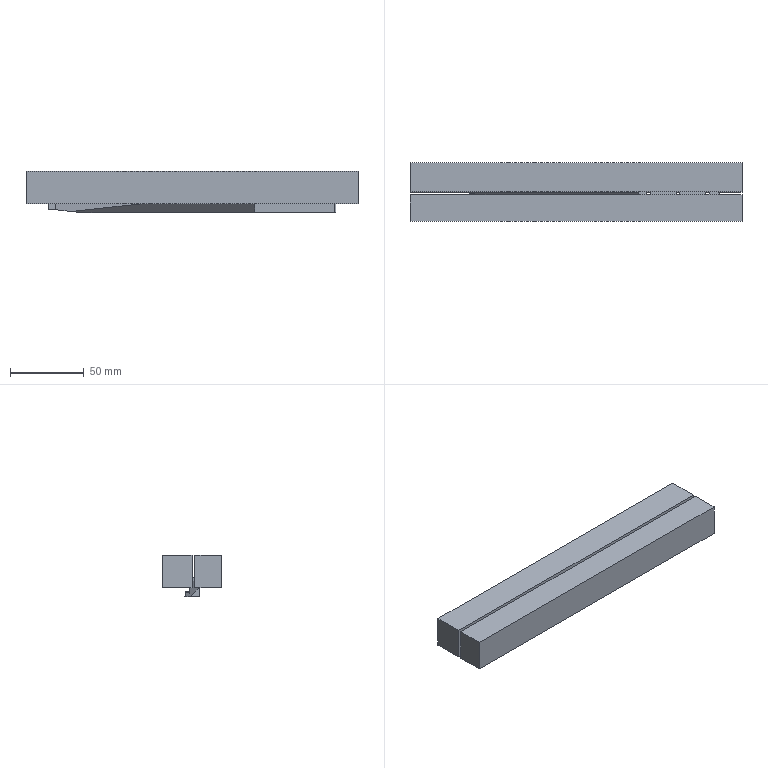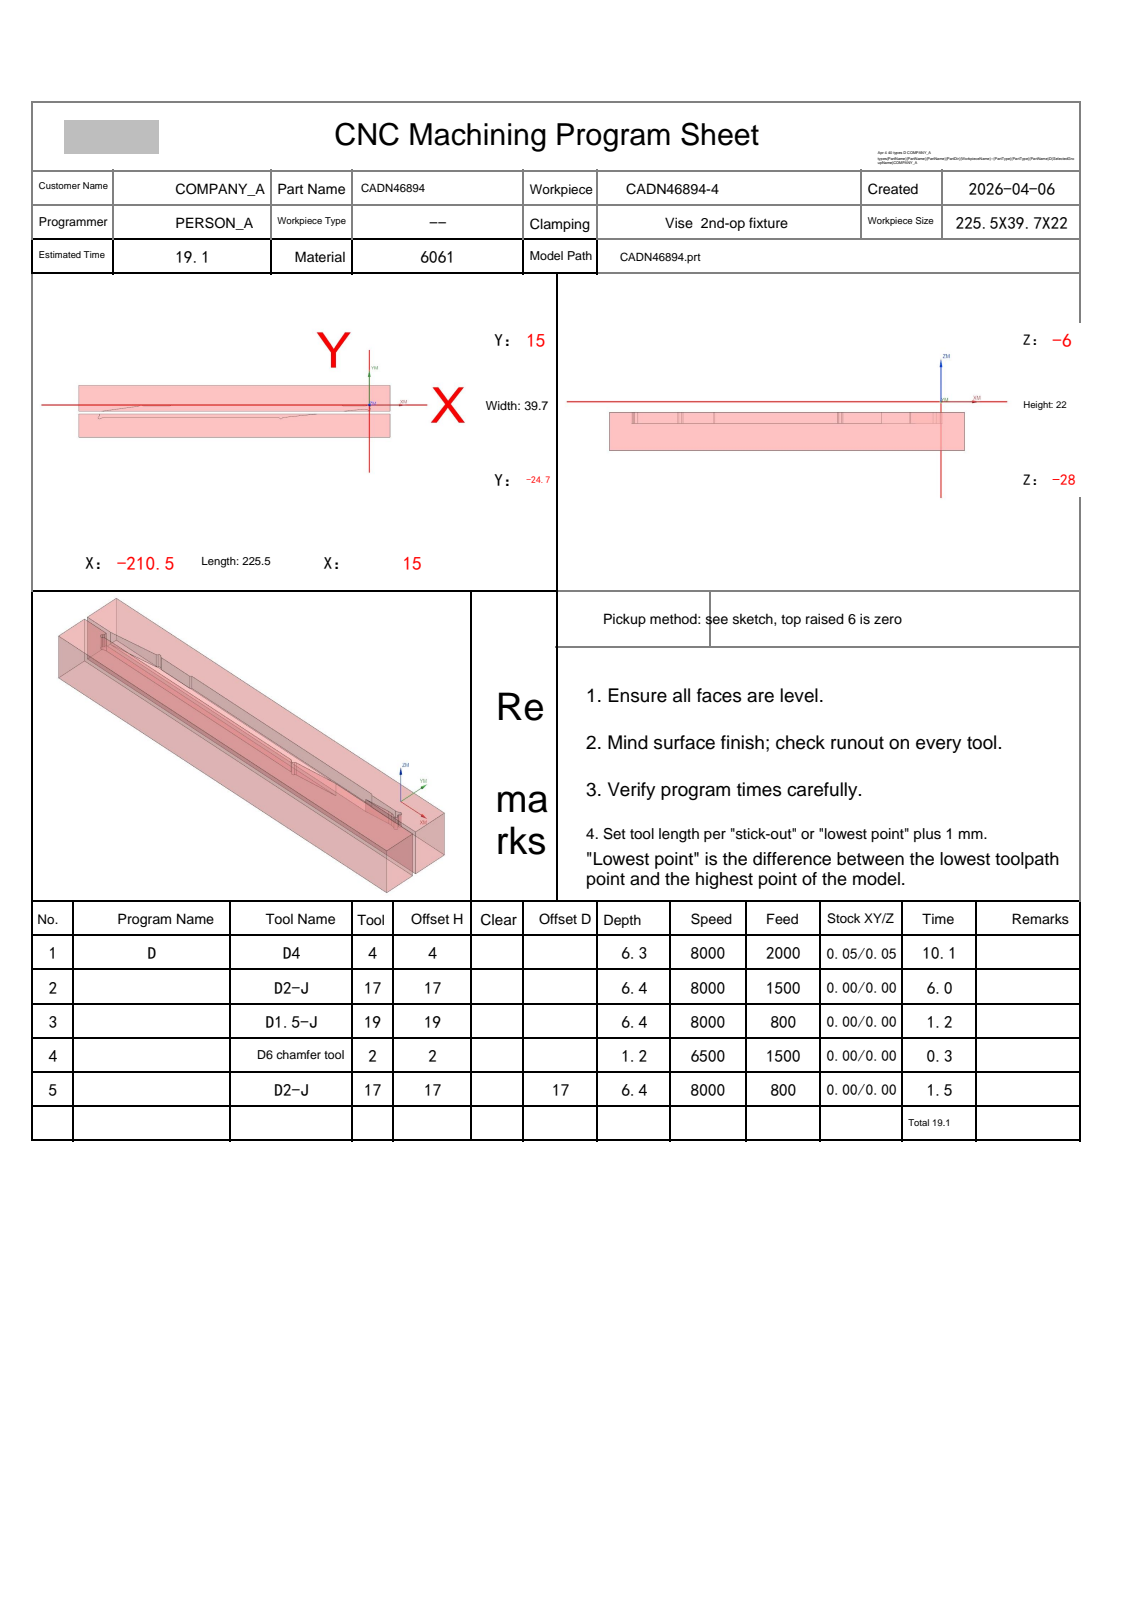NC program | NX | posted by the shop | part box 225.5 x 39.7 x 28 mm
Lines 1 to 1400 of 3483:
%
O0001
(Machine time: 204.82 MIN)
(===Total Tool:8===)
(T9=D10     D=10.  R=0.   D-  H09 Z=-13.1 )
(T2=D6 chamfer tool   D=6.   R=0.   D-  H02 Z=-2.05 )
(T12=ZT2.5  D=2.5  DR_a=118 D-  H12 Z=-18.45)
(T20=M3X0.5 D=2.5  DR_a=180 D-  H20 Z=-15.7 )
(T4=D4      D=4.   R=0.   D-  H04 Z=-6.   )
(T7=D6-J    D=6.   R=0.   D7  H07 Z=-13.1 )
(T17=D2-J   D=2.   R=0.   D-  H17 Z=-5.9  )
(T18=D4R0.5 D=4.   R=0.5  D-  H18 Z=-6.51 )
G80 G90 G17 G49 G40
G91 G28 Z0
M01
N1 T09 M06
(D10  D=10. R=0. H=09 ce=0.10 di=0.10)
G00 G90 G54 X-99.772 Y-4.501 M03 S8000
G43 H09 Z20.
M08
Z.7
G01 X-100.447 Y-4.214 Z.662 F4000.
X-101.626 Y-3.21 Z.58
X-102.452 Y-1.901 Z.499
X-102.85 Y-.404 Z.418
Y4.404 Z.166
X-102.49 Y5.813 Z.09
X-101.748 Y7.065 Z.014
X-99.965 Y8.848 Z-.119
X-98.713 Y9.59 Z-.195
X-97.304 Y9.95 Z-.271
X-96.75 Z-.3
X34.026 Z-.477
X93.026 Y3.55 Z-.557
X97.25 Z-.563
G02 X102.85 Y-2.05 Z-.575 I0.0 J-5.6
G01 Y-3.65 Z-.577
G02 X97.25 Y-9.25 Z-.589 I-5.6 J0.0
G01 X77.329 Z-.616
G02 X74.75 Y-9.95 Z-.619 I-2.579 J4.4
G01 X-42.75 Z-.778
G02 X-45.329 Y-9.25 Z-.782 I0.0 J5.1
G01 X-68.114 Z-.813
X-98.474 Y-4.898 Z-.854
G02 X-102.85 Y.15 Z-.864 I.724 J5.048
G01 Y3.85 Z-.869
G02 X-101.356 Y7.456 Z-.874 I5.1 J0.0
G01 X-100.356 Y8.456 Z-.876
G02 X-96.75 Y9.95 Z-.882 I3.606 J-3.606
G01 X34.026 Z-1.059
X93.026 Y3.55 Z-1.139
X97.25 Z-1.145
G02 X102.85 Y-2.05 Z-1.157 I0.0 J-5.6
G01 Y-3.65 Z-1.159
G02 X97.25 Y-9.25 Z-1.171 I-5.6 J0.0
G01 X77.329 Z-1.198
G02 X74.75 Y-9.95 Z-1.201 I-2.579 J4.4
G01 X-42.75 Z-1.36
G02 X-45.329 Y-9.25 Z-1.364 I0.0 J5.1
G01 X-68.114 Z-1.395
X-98.474 Y-4.898 Z-1.436
G02 X-102.85 Y.15 Z-1.446 I.724 J5.048
G01 Y3.85 Z-1.451
G02 X-101.356 Y7.456 Z-1.456 I5.1 J0.0
G01 X-100.356 Y8.456 Z-1.458
G02 X-96.75 Y9.95 Z-1.464 I3.606 J-3.606
G01 X34.026 Z-1.64
X93.026 Y3.55 Z-1.721
X97.25 Z-1.726
G02 X102.85 Y-2.05 Z-1.738 I0.0 J-5.6
G01 Y-3.65 Z-1.741
G02 X97.25 Y-9.25 Z-1.752 I-5.6 J0.0
G01 X77.329 Z-1.779
G02 X74.75 Y-9.95 Z-1.783 I-2.579 J4.4
G01 X-42.75 Z-1.942
G02 X-45.329 Y-9.25 Z-1.946 I0.0 J5.1
G01 X-68.114 Z-1.976
X-98.474 Y-4.898 Z-2.018
G02 X-102.85 Y.15 Z-2.028 I.724 J5.048
G01 Y3.85 Z-2.033
G02 X-101.356 Y7.456 Z-2.038 I5.1 J0.0
G01 X-100.356 Y8.456 Z-2.04
G02 X-96.75 Y9.95 Z-2.045 I3.606 J-3.606
G01 X34.026 Z-2.222
X93.026 Y3.55 Z-2.303
X97.25 Z-2.308
G02 X102.85 Y-2.05 Z-2.32 I0.0 J-5.6
G01 Y-3.65 Z-2.322
G02 X97.25 Y-9.25 Z-2.334 I-5.6 J0.0
G01 X77.329 Z-2.361
G02 X74.75 Y-9.95 Z-2.365 I-2.579 J4.4
G01 X-42.75 Z-2.524
G02 X-45.329 Y-9.25 Z-2.527 I0.0 J5.1
G01 X-68.114 Z-2.558
X-98.474 Y-4.898 Z-2.6
G02 X-102.85 Y.15 Z-2.61 I.724 J5.048
G01 Y3.85 Z-2.615
G02 X-101.356 Y7.456 Z-2.62 I5.1 J0.0
G01 X-100.356 Y8.456 Z-2.622
G02 X-96.75 Y9.95 Z-2.627 I3.606 J-3.606
G01 X34.026 Z-2.804
X93.026 Y3.55 Z-2.884
X97.25 Z-2.89
G02 X102.85 Y-2.05 Z-2.902 I0.0 J-5.6
G01 Y-3.65 Z-2.904
G02 X97.25 Y-9.25 Z-2.916 I-5.6 J0.0
G01 X77.329 Z-2.943
G02 X74.75 Y-9.95 Z-2.947 I-2.579 J4.4
G01 X-42.75 Z-3.106
G02 X-45.329 Y-9.25 Z-3.109 I0.0 J5.1
G01 X-68.114 Z-3.14
X-98.474 Y-4.898 Z-3.181
G02 X-102.85 Y.15 Z-3.191 I.724 J5.048
G01 Y3.85 Z-3.196
G02 X-101.356 Y7.456 Z-3.202 I5.1 J0.0
G01 X-100.356 Y8.456 Z-3.204
G02 X-96.75 Y9.95 Z-3.209 I3.606 J-3.606
G01 X34.026 Z-3.386
X93.026 Y3.55 Z-3.466
X97.25 Z-3.472
G02 X102.85 Y-2.05 Z-3.484 I0.0 J-5.6
G01 Y-3.65 Z-3.486
G02 X97.25 Y-9.25 Z-3.498 I-5.6 J0.0
G01 X77.329 Z-3.525
G02 X74.75 Y-9.95 Z-3.528 I-2.579 J4.4
G01 X-42.75 Z-3.687
G02 X-45.329 Y-9.25 Z-3.691 I0.0 J5.1
G01 X-68.114 Z-3.722
X-98.474 Y-4.898 Z-3.763
G02 X-102.85 Y.15 Z-3.773 I.724 J5.048
G01 Y3.85 Z-3.778
G02 X-101.356 Y7.456 Z-3.784 I5.1 J0.0
G01 X-100.356 Y8.456 Z-3.785
G02 X-96.75 Y9.95 Z-3.791 I3.606 J-3.606
G01 X34.026 Z-3.968
X93.026 Y3.55 Z-4.048
X97.25 Z-4.054
G02 X102.85 Y-2.05 Z-4.066 I0.0 J-5.6
G01 Y-3.65 Z-4.068
G02 X97.25 Y-9.25 Z-4.08 I-5.6 J0.0
G01 X77.329 Z-4.107
G02 X74.75 Y-9.95 Z-4.11 I-2.579 J4.4
G01 X-42.75 Z-4.269
G02 X-45.329 Y-9.25 Z-4.273 I0.0 J5.1
G01 X-68.114 Z-4.304
X-98.474 Y-4.898 Z-4.345
G02 X-102.85 Y.15 Z-4.355 I.724 J5.048
G01 Y3.85 Z-4.36
G02 X-101.356 Y7.456 Z-4.365 I5.1 J0.0
G01 X-100.356 Y8.456 Z-4.367
G02 X-96.75 Y9.95 Z-4.373 I3.606 J-3.606
G01 X34.026 Z-4.55
X93.026 Y3.55 Z-4.63
X97.25 Z-4.636
G02 X102.85 Y-2.05 Z-4.647 I0.0 J-5.6
G01 Y-3.65 Z-4.65
G02 X97.25 Y-9.25 Z-4.662 I-5.6 J0.0
G01 X77.329 Z-4.688
G02 X74.75 Y-9.95 Z-4.692 I-2.579 J4.4
G01 X-42.75 Z-4.851
G02 X-45.329 Y-9.25 Z-4.855 I0.0 J5.1
G01 X-68.114 Z-4.885
X-98.474 Y-4.898 Z-4.927
G02 X-102.85 Y.15 Z-4.937 I.724 J5.048
G01 Y3.85 Z-4.942
G02 X-101.356 Y7.456 Z-4.947 I5.1 J0.0
G01 X-100.356 Y8.456 Z-4.949
G02 X-96.75 Y9.95 Z-4.955 I3.606 J-3.606
G01 X34.026 Z-5.131
X93.026 Y3.55 Z-5.212
X97.25 Z-5.217
G02 X102.85 Y-2.05 Z-5.229 I0.0 J-5.6
G01 Y-3.65 Z-5.231
G02 X97.25 Y-9.25 Z-5.243 I-5.6 J0.0
G01 X77.329 Z-5.27
G02 X74.75 Y-9.95 Z-5.274 I-2.579 J4.4
G01 X-42.75 Z-5.433
G02 X-45.329 Y-9.25 Z-5.436 I0.0 J5.1
G01 X-68.114 Z-5.467
X-98.474 Y-4.898 Z-5.509
G02 X-102.85 Y.15 Z-5.519 I.724 J5.048
G01 Y3.85 Z-5.524
G02 X-101.356 Y7.456 Z-5.529 I5.1 J0.0
G01 X-100.356 Y8.456 Z-5.531
G02 X-96.75 Y9.95 Z-5.536 I3.606 J-3.606
G01 X34.026 Z-5.713
X93.026 Y3.55 Z-5.793
X97.25 Z-5.799
G02 X102.85 Y-2.05 Z-5.811 I0.0 J-5.6
G01 Y-3.65 Z-5.813
G02 X97.25 Y-9.25 Z-5.825 I-5.6 J0.0
G01 X77.329 Z-5.852
G02 X74.75 Y-9.95 Z-5.856 I-2.579 J4.4
G01 X-42.75 Z-6.015
G02 X-45.329 Y-9.25 Z-6.018 I0.0 J5.1
G01 X-68.114 Z-6.049
X-98.474 Y-4.898 Z-6.091
G02 X-102.85 Y.15 Z-6.1 I.724 J5.048
G01 Y3.85 Z-6.105
G02 X-101.356 Y7.456 Z-6.111 I5.1 J0.0
G01 X-100.356 Y8.456 Z-6.113
G02 X-96.75 Y9.95 Z-6.118 I3.606 J-3.606
G01 X34.026 Z-6.295
X93.026 Y3.55 Z-6.375
X97.25 Z-6.381
G02 X102.85 Y-2.05 Z-6.393 I0.0 J-5.6
G01 Y-3.65 Z-6.395
G02 X97.25 Y-9.25 Z-6.407 I-5.6 J0.0
G01 X77.329 Z-6.434
G02 X74.75 Y-9.95 Z-6.438 I-2.579 J4.4
G01 X-42.75 Z-6.596
G02 X-45.329 Y-9.25 Z-6.6 I0.0 J5.1
G01 X-68.114 Z-6.631
X-98.474 Y-4.898 Z-6.672
G02 X-102.85 Y.15 Z-6.682 I.724 J5.048
G01 Y3.85 Z-6.687
G02 X-101.356 Y7.456 Z-6.693 I5.1 J0.0
G01 X-100.356 Y8.456 Z-6.695
G02 X-96.75 Y9.95 Z-6.7 I3.606 J-3.606
G01 X34.026 Z-6.877
X93.026 Y3.55 Z-6.957
X97.25 Z-6.963
G02 X102.85 Y-2.05 Z-6.975 I0.0 J-5.6
G01 Y-3.65 Z-6.977
G02 X97.25 Y-9.25 Z-6.989 I-5.6 J0.0
G01 X77.329 Z-7.016
G02 X74.75 Y-9.95 Z-7.019 I-2.579 J4.4
G01 X-42.75 Z-7.178
G02 X-45.329 Y-9.25 Z-7.182 I0.0 J5.1
G01 X-68.114 Z-7.213
X-98.474 Y-4.898 Z-7.254
G02 X-102.85 Y.15 Z-7.264 I.724 J5.048
G01 Y3.85 Z-7.269
G02 X-101.356 Y7.456 Z-7.274 I5.1 J0.0
G01 X-100.356 Y8.456 Z-7.276
G02 X-96.75 Y9.95 Z-7.282 I3.606 J-3.606
G01 X34.026 Z-7.459
X93.026 Y3.55 Z-7.539
X97.25 Z-7.545
G02 X102.85 Y-2.05 Z-7.557 I0.0 J-5.6
G01 Y-3.65 Z-7.559
G02 X97.25 Y-9.25 Z-7.571 I-5.6 J0.0
G01 X77.329 Z-7.598
G02 X74.75 Y-9.95 Z-7.601 I-2.579 J4.4
G01 X-42.75 Z-7.76
G02 X-45.329 Y-9.25 Z-7.764 I0.0 J5.1
G01 X-68.114 Z-7.795
X-98.474 Y-4.898 Z-7.836
G02 X-102.85 Y.15 Z-7.846 I.724 J5.048
G01 Y3.85 Z-7.851
G02 X-101.356 Y7.456 Z-7.856 I5.1 J0.0
G01 X-100.356 Y8.456 Z-7.858
G02 X-96.75 Y9.95 Z-7.864 I3.606 J-3.606
G01 X34.026 Z-8.04
X93.026 Y3.55 Z-8.121
X97.25 Z-8.126
G02 X102.85 Y-2.05 Z-8.138 I0.0 J-5.6
G01 Y-3.65 Z-8.141
G02 X97.25 Y-9.25 Z-8.152 I-5.6 J0.0
G01 X77.329 Z-8.179
G02 X74.75 Y-9.95 Z-8.183 I-2.579 J4.4
G01 X-42.75 Z-8.342
G02 X-45.329 Y-9.25 Z-8.346 I0.0 J5.1
G01 X-68.114 Z-8.376
X-98.474 Y-4.898 Z-8.418
G02 X-102.85 Y.15 Z-8.428 I.724 J5.048
G01 Y3.85 Z-8.433
G02 X-101.356 Y7.456 Z-8.438 I5.1 J0.0
G01 X-100.356 Y8.456 Z-8.44
G02 X-96.75 Y9.95 Z-8.445 I3.606 J-3.606
G01 X34.026 Z-8.622
X93.026 Y3.55 Z-8.703
X97.25 Z-8.708
G02 X102.85 Y-2.05 Z-8.72 I0.0 J-5.6
G01 Y-3.65 Z-8.722
G02 X97.25 Y-9.25 Z-8.734 I-5.6 J0.0
G01 X77.329 Z-8.761
G02 X74.75 Y-9.95 Z-8.765 I-2.579 J4.4
G01 X-42.75 Z-8.924
G02 X-45.329 Y-9.25 Z-8.927 I0.0 J5.1
G01 X-68.114 Z-8.958
X-98.474 Y-4.898 Z-9.
G02 X-102.85 Y.15 Z-9.01 I.724 J5.048
G01 Y3.85 Z-9.015
G02 X-101.356 Y7.456 Z-9.02 I5.1 J0.0
G01 X-100.356 Y8.456 Z-9.022
G02 X-96.75 Y9.95 Z-9.027 I3.606 J-3.606
G01 X34.026 Z-9.204
X93.026 Y3.55 Z-9.284
X97.25 Z-9.29
G02 X102.85 Y-2.05 Z-9.302 I0.0 J-5.6
G01 Y-3.65 Z-9.304
G02 X97.25 Y-9.25 Z-9.316 I-5.6 J0.0
G01 X77.329 Z-9.343
G02 X74.75 Y-9.95 Z-9.347 I-2.579 J4.4
G01 X-42.75 Z-9.506
G02 X-45.329 Y-9.25 Z-9.509 I0.0 J5.1
G01 X-68.114 Z-9.54
X-98.474 Y-4.898 Z-9.581
G02 X-102.85 Y.15 Z-9.591 I.724 J5.048
G01 Y3.85 Z-9.596
G02 X-101.356 Y7.456 Z-9.602 I5.1 J0.0
G01 X-100.356 Y8.456 Z-9.604
G02 X-96.75 Y9.95 Z-9.609 I3.606 J-3.606
G01 X34.026 Z-9.786
X93.026 Y3.55 Z-9.866
X97.25 Z-9.872
G02 X102.85 Y-2.05 Z-9.884 I0.0 J-5.6
G01 Y-3.65 Z-9.886
G02 X97.25 Y-9.25 Z-9.898 I-5.6 J0.0
G01 X77.329 Z-9.925
G02 X74.75 Y-9.95 Z-9.928 I-2.579 J4.4
G01 X-42.75 Z-10.087
G02 X-45.329 Y-9.25 Z-10.091 I0.0 J5.1
G01 X-68.114 Z-10.122
X-98.474 Y-4.898 Z-10.163
G02 X-102.85 Y.15 Z-10.173 I.724 J5.048
G01 Y3.85 Z-10.178
G02 X-101.356 Y7.456 Z-10.184 I5.1 J0.0
G01 X-100.356 Y8.456 Z-10.185
G02 X-96.75 Y9.95 Z-10.191 I3.606 J-3.606
G01 X34.026 Z-10.368
X93.026 Y3.55 Z-10.448
X97.25 Z-10.454
G02 X102.85 Y-2.05 Z-10.466 I0.0 J-5.6
G01 Y-3.65 Z-10.468
G02 X97.25 Y-9.25 Z-10.48 I-5.6 J0.0
G01 X77.329 Z-10.507
G02 X74.75 Y-9.95 Z-10.51 I-2.579 J4.4
G01 X-42.75 Z-10.669
G02 X-45.329 Y-9.25 Z-10.673 I0.0 J5.1
G01 X-68.114 Z-10.704
X-98.474 Y-4.898 Z-10.745
G02 X-102.85 Y.15 Z-10.755 I.724 J5.048
G01 Y3.85 Z-10.76
G02 X-101.356 Y7.456 Z-10.765 I5.1 J0.0
G01 X-100.356 Y8.456 Z-10.767
G02 X-96.75 Y9.95 Z-10.773 I3.606 J-3.606
G01 X34.026 Z-10.95
X93.026 Y3.55 Z-11.03
X97.25 Z-11.036
G02 X102.85 Y-2.05 Z-11.047 I0.0 J-5.6
G01 Y-3.65 Z-11.05
G02 X97.25 Y-9.25 Z-11.062 I-5.6 J0.0
G01 X77.329 Z-11.088
G02 X74.75 Y-9.95 Z-11.092 I-2.579 J4.4
G01 X-42.75 Z-11.251
G02 X-45.329 Y-9.25 Z-11.255 I0.0 J5.1
G01 X-68.114 Z-11.285
X-98.474 Y-4.898 Z-11.327
G02 X-102.85 Y.15 Z-11.337 I.724 J5.048
G01 Y3.85 Z-11.342
G02 X-101.356 Y7.456 Z-11.347 I5.1 J0.0
G01 X-100.356 Y8.456 Z-11.349
G02 X-96.75 Y9.95 Z-11.355 I3.606 J-3.606
G01 X34.026 Z-11.531
X93.026 Y3.55 Z-11.612
X97.25 Z-11.617
G02 X102.85 Y-2.05 Z-11.629 I0.0 J-5.6
G01 Y-3.65 Z-11.631
G02 X97.25 Y-9.25 Z-11.643 I-5.6 J0.0
G01 X77.329 Z-11.67
G02 X74.75 Y-9.95 Z-11.674 I-2.579 J4.4
G01 X-42.75 Z-11.833
G02 X-45.329 Y-9.25 Z-11.836 I0.0 J5.1
G01 X-68.114 Z-11.867
X-98.474 Y-4.898 Z-11.909
G02 X-102.85 Y.15 Z-11.919 I.724 J5.048
G01 Y3.85 Z-11.924
G02 X-101.356 Y7.456 Z-11.929 I5.1 J0.0
G01 X-100.356 Y8.456 Z-11.931
G02 X-96.75 Y9.95 Z-11.936 I3.606 J-3.606
G01 X34.026 Z-12.113
X93.026 Y3.55 Z-12.193
X97.25 Z-12.199
G02 X102.85 Y-2.05 Z-12.211 I0.0 J-5.6
G01 Y-3.65 Z-12.213
G02 X97.25 Y-9.25 Z-12.225 I-5.6 J0.0
G01 X77.329 Z-12.252
G02 X74.75 Y-9.95 Z-12.256 I-2.579 J4.4
G01 X-42.75 Z-12.415
G02 X-45.329 Y-9.25 Z-12.418 I0.0 J5.1
G01 X-68.114 Z-12.449
X-98.474 Y-4.898 Z-12.491
G02 X-102.85 Y.15 Z-12.5 I.724 J5.048
G01 Y3.85 Z-12.505
G02 X-101.356 Y7.456 Z-12.511 I5.1 J0.0
G01 X-100.356 Y8.456 Z-12.513
G02 X-96.75 Y9.95 Z-12.518 I3.606 J-3.606
G01 X34.026 Z-12.695
X93.026 Y3.55 Z-12.775
X97.25 Z-12.781
G02 X102.85 Y-2.05 Z-12.793 I0.0 J-5.6
G01 Y-3.65 Z-12.795
G02 X97.25 Y-9.25 Z-12.807 I-5.6 J0.0
G01 X77.329 Z-12.834
G02 X74.75 Y-9.95 Z-12.838 I-2.579 J4.4
G01 X-42.75 Z-12.996
G02 X-45.329 Y-9.25 Z-13. I0.0 J5.1
G01 X-68.114 Z-13.031
X-98.474 Y-4.898 Z-13.072
G02 X-102.85 Y.15 Z-13.082 I.724 J5.048
G01 Y3.85 Z-13.087
G02 X-101.356 Y7.456 Z-13.093 I5.1 J0.0
G01 X-100.356 Y8.456 Z-13.095
G02 X-96.75 Y9.95 Z-13.1 I3.606 J-3.606
G01 X34.026
X93.026 Y3.55
X97.25
G02 X102.85 Y-2.05 I0.0 J-5.6
G01 Y-3.65
G02 X97.25 Y-9.25 I-5.6 J0.0
G01 X77.329
G02 X74.75 Y-9.95 I-2.579 J4.4
G01 X-42.75
G02 X-45.329 Y-9.25 I0.0 J5.1
G01 X-68.114
X-98.474 Y-4.898
G02 X-102.85 Y.15 I.724 J5.048
G01 Y3.85
G02 X-101.356 Y7.456 I5.1 J0.0
G01 X-100.356 Y8.456
G02 X-96.75 Y9.95 I3.606 J-3.606
G01 X-96.35
Z-12.1
G00 Z20.
G00 G90 X-99.94 Y12.625 M03 S8000
Z10.2
Z1.3
G01 Z-.2 F4000.
X-100.276 Y8.254
G03 X-100.43 Y4.23 I52.346 J-4.024
G01 Y-3.549
G03 X-99.572 Y-4.539 I1. J0.0
G01 X-93.843 Y-5.36
X-93.73 Y-5.368
G03 X-92.93 Y-4.568 I0.0 J.8
G01 Y4.23
G02 X-92.692 Y8.853 I45. J0.0
X-91.698 Y9.75 I.995 J-.103
G01 X-85.938
G02 X-85.138 Y8.95 I0.0 J-.8
G01 X-85.144 Y8.852
G03 X-85.43 Y4.23 I37.214 J-4.622
G01 Y-5.699
G03 X-84.572 Y-6.689 I1. J0.0
G01 X-78.843 Y-7.51
X-78.73 Y-7.518
G03 X-77.93 Y-6.718 I0.0 J.8
G01 Y4.23
G02 X-77.563 Y8.906 I30. J0.0
X-76.576 Y9.75 I.988 J-.156
G01 X-70.623
G02 X-69.924 Y9.05 I0.0 J-.7
G01 X-69.939 Y8.905
G03 X-70.43 Y4.23 I22.009 J-4.675
G01 Y-7.849
G03 X-69.572 Y-8.839 I1. J0.0
G01 X-68.17 Y-9.04
X-68.028 Y-9.05
X-63.93
G03 X-62.93 Y-8.05 I0.0 J1.
G01 Y4.23
G02 X-62.127 Y9.073 I15. J0.0
X-61.181 Y9.75 I.946 J-.323
G01 X-53.946
G02 X-53.546 Y9.35 I0.0 J-.4
X-53.642 Y9.091 I-.4 J0.0
G03 X-55.43 Y4.23 I5.712 J-4.861
G01 Y-8.194
G03 X-54.584 Y-9.182 I1. J0.0
G01 X-49.084 Y-10.038
X-48.93 Y-10.05
G03 X-47.93 Y-9.05 I0.0 J1.
G01 Y4.23
X-37.85
X-34.85
X-34.75 Y7.23
Z1.3
G00 Z10.2
G91 G28 Z0.0
M05
M09
G91 G28 Z0.0
M01
N2 T02 M06
(D6 chamfer tool  D=6. R=0. H=02 ce=0.00 di=0.10)
G00 G90 G54 X-89.25 Y.85 M03 S8000
G43 H02 Z20.
M08
G98 G81 X-89.25 Y.85 Z-1.1 R.7 F500.
X-69.25
X-49.25
G80
G00 Z20.
G91 G28 Z0.0
M05
M09
G91 G28 Z0.0
M01
N3 T12 M06
(ZT2.5 D=2.5 DR_a=118 H=12)
G00 G90 G54 X-89.25 Y.85 M03 S3000
G43 H12 Z20.
M08
G98 G83 X-89.25 Y.85 Z-18.451 R.7 F300. Q2.
X-69.25
X-49.25
G80
G00 Z20.
G91 G28 Z0.0
M05
M09
G91 G28 Z0.0
M01
N4 T02 M06
(D6 chamfer tool  D=6. R=0. H=02 ce=0.00 di=0.10)
G00 G90 G54 X-89.25 Y.85 M03 S8000
G43 H02 Z20.
M08
G98 G81 X-89.25 Y.85 Z-2.05 R2.7 F500.
X-69.25
X-49.25
G80
G00 Z20.
G91 G28 Z0.0
M05
M09
G91 G28 Z0.0
M01
N5 T20 M06
(M3X0.5 D=2.5 DR_a=180 H=20)
G00 G90 G54 X-89.25 Y.85 M03 S800
G43 H20 Z20.
M08
G95
G98 G84 X-89.25 Y.85 Z-15.7 R.7 F.5 Q5.
X-69.25
X-49.25
G80
G94
G00 Z20.
G91 G28 Z0.0
M05
M09
G91 G28 Z0.0
M01
N6 T04 M06
(D4  D=4. R=0. H=04 ce=0.10 di=0.10)
G00 G90 G54 X3.822 Y9.801 M03 S8000
G43 H04 Z10.2
M08
Z.9
G01 Z-.3 F2000.
Y9.35
G03 X6.622 Y6.55 I2.8 J0.0
G01 X37.906
X38.366 Y6.5
X81.179 Y1.851
X85.196 Y1.415
G02 X86.565 Y.891 I-.486 J-3.321
X87.43 Y-.678 I-2.64 J-2.478
G01 X87.532 Y-.69
X94.779 Y-1.471
X99.273 Y-1.468
X99.305 Y-1.475
X99.749 Y-1.663
X99.815 Y-1.667
X99.797 Y-1.731
X99.814 Y-1.948
X99.834 Y-2.509
Y-3.624
X99.829 Y-3.651
X99.643 Y-4.167
X99.637 Y-4.238
X99.568 Y-4.22
X98.16 Y-4.23
X86.972 Y-4.229
X86.974 Y-.75
G03 X84.849 Y1.291 I-2.126 J-.086
G01 X-40.65
Y4.739
X-40.648 Y4.837
G03 X-42.401 Y6.922 I-2.116 J0.0
G01 X-42.397 Y6.947
X-42.374 Y6.981
X-42.321 Y7.001
X-41.189
G02 X-40.708 Y6.55 I-1.575 J-2.164
G01 X7.557
G02 X7.839 Y6.433 I0.0 J-.4
G01 X9.405 Y4.867
G03 X9.688 Y4.75 I.283 J.283
G01 X37.829 Y4.748
X38.171 Y4.711
X51.615 Y3.251
X51.686 Y3.171
X51.607 Y3.091
X-38.452
G02 X-38.85 Y3.49 I.002 J.4
G01 Y4.352
G02 X-38.452 Y4.75 I.4 J-.002
G01 X8.622
X9.122
G03 X11.922 Y7.55 I0.0 J2.8
G01 Y9.801
Z.9
G00 Z3.
G01 X2.433 F6000.
G00 Z.6
G01 Z-.6 F2000.
Y9.35
G03 X5.233 Y6.55 I2.8 J0.0
G01 X37.906
X38.366 Y6.5
X49.047 Y5.34
X85.196 Y1.415
G02 X85.551 Y1.344 I-.481 J-3.322
G01 X85.556 Y1.343
X83.811 Y1.532
X82.88 Y1.591
X-40.65
Y4.739
X-40.648 Y4.837
G03 X-40.686 Y5.237 I-2.116 J0.0
X-42.258 Y6.892 I-2.064 J-.387
G01 X-42.401 Y6.922
X-42.397 Y6.947
X-42.374 Y6.981
X-42.321 Y7.001
X-41.185
G02 X-40.704 Y6.55 I-1.565 J-2.151
G01 X7.233
G02 X7.611 Y6.279 I0.0 J-.4
G01 X8.041 Y5.021
G03 X8.419 Y4.75 I.379 J.129
G01 X37.828 Y4.748
X38.171 Y4.711
X48.853 Y3.551
X48.923 Y3.471
X48.844 Y3.391
X-38.452
G02 X-38.85 Y3.79 I.002 J.4
G01 Y4.352
G02 X-38.452 Y4.75 I.4 J-.002
G01 X7.233
X7.733
G03 X10.533 Y7.55 I0.0 J2.8
G01 Y9.801
Z.6
G00 Z2.7
G01 X1.043 F6000.
G00 Z.3
G01 Z-.9 F2000.
Y9.35
G03 X3.843 Y6.55 I2.8 J0.0
G01 X37.906
X38.366 Y6.5
X80.082 Y1.97
X85.196 Y1.415
G02 X85.556 Y1.343 I-.481 J-3.322
G01 X83.811 Y1.532
X80.992 Y1.838
X80.074 Y1.891
X-40.65
Y4.739
X-40.648 Y4.837
G03 X-40.686 Y5.237 I-2.116 J0.0
X-42.258 Y6.892 I-2.064 J-.387
G01 X-42.401 Y6.922
X-42.397 Y6.947
X-42.374 Y6.981
X-42.321 Y7.001
X-41.185
G02 X-40.704 Y6.55 I-1.565 J-2.151
G01 X5.843
G02 X6.222 Y6.279 I0.0 J-.4
G01 X6.651 Y5.021
G03 X7.029 Y4.75 I.379 J.129
G01 X37.828 Y4.748
X38.171 Y4.711
X46.09 Y3.851
X46.16 Y3.771
X46.081 Y3.691
X-38.452
G02 X-38.85 Y4.09 I.002 J.4
G01 Y4.352
G02 X-38.452 Y4.75 I.4 J-.002
G01 X5.843
X6.343
G03 X9.143 Y7.55 I0.0 J2.8
G01 Y9.801
Z.3
G00 Z2.4
G01 X-.366 F6000.
G00 Z0.0
G01 Z-1.2 F2000.
Y9.35
G03 X2.434 Y6.55 I2.8 J0.0
G01 X37.906
X38.366 Y6.5
X77.319 Y2.27
X85.196 Y1.415
G02 X85.556 Y1.343 I-.481 J-3.322
G01 X78.226 Y2.138
X77.348 Y2.191
X-40.65
Y4.739
X-40.648 Y4.837
G03 X-40.686 Y5.237 I-2.116 J0.0
X-42.258 Y6.892 I-2.064 J-.387
G01 X-42.401 Y6.922
X-42.397 Y6.947
X-42.374 Y6.981
X-42.321 Y7.001
X-41.185
G02 X-40.704 Y6.55 I-1.565 J-2.151
G01 X4.434
G02 X4.812 Y6.279 I0.0 J-.4
G01 X5.241 Y5.021
G03 X5.62 Y4.75 I.378 J.129
G01 X37.826 Y4.748
X38.171 Y4.711
X43.327 Y4.151
X43.397 Y4.071
X43.318 Y3.991
X-38.492
G02 X-38.852 Y4.354 I.002 J.362
G01 X-38.85 Y4.392
G02 X-38.492 Y4.75 I.36 J-.002
G01 X4.434
X4.934
G03 X7.734 Y7.55 I0.0 J2.8
G01 Y9.801
Z0.0
G00 Z2.1
G01 X-1.836 F6000.
G00 Z-.3
G01 Z-1.5 F2000.
Y9.35
G03 X.964 Y6.55 I2.8 J0.0
G01 X37.906
X38.366 Y6.5
X70.127 Y3.051
X74.556 Y2.57
X85.196 Y1.415
G02 X85.556 Y1.343 I-.481 J-3.322
G01 X75.461 Y2.438
X74.583 Y2.491
X-40.65
Y4.739
X-40.648 Y4.837
G03 X-40.686 Y5.237 I-2.116 J0.0
X-42.258 Y6.892 I-2.064 J-.387
G01 X-42.401 Y6.922
X-42.397 Y6.947
X-42.374 Y6.981
X-42.321 Y7.001
X-41.185
G02 X-40.704 Y6.55 I-1.565 J-2.151
G01 X2.964
G02 X3.343 Y6.279 I0.0 J-.4
G01 X3.772 Y5.021
G03 X4.15 Y4.75 I.378 J.129
G01 X37.818 Y4.749
X38.171 Y4.711
X40.564 Y4.451
X40.635 Y4.371
X40.556 Y4.291
X-38.652
G02 X-38.85 Y4.49 I.002 J.2
G01 Y4.552
G02 X-38.652 Y4.75 I.2 J-.002
G01 X2.964
X3.464
G03 X6.264 Y7.55 I0.0 J2.8
G01 Y9.801
Z-.3
G00 Z1.8
G01 X12.844 F6000.
G00 Z-.6
G01 Z-1.8 F2000.
Y9.35
G03 X15.644 Y6.55 I2.8 J0.0
G01 X37.906
X38.366 Y6.5
X71.794 Y2.87
X85.196 Y1.415
G02 X85.556 Y1.343 I-.481 J-3.322
G01 X72.695 Y2.738
X71.785 Y2.791
X-40.65
Y4.739
X-40.648 Y4.837
G03 X-40.686 Y5.237 I-2.116 J0.0
X-42.258 Y6.892 I-2.064 J-.387
G01 X-42.401 Y6.922
X-42.397 Y6.947
X-42.374 Y6.981
X-42.321 Y7.001
X-41.185
G02 X-40.704 Y6.55 I-1.565 J-2.151
G01 X15.644
X16.144
G03 X18.944 Y9.35 I0.0 J2.8
G01 Y9.801
Z-.6
G00 Z1.5
G01 X11.454 F6000.
G00 Z-.9
G01 Z-2.1 F2000.
Y9.35
G03 X14.254 Y6.55 I2.8 J0.0
G01 X37.906
X38.366 Y6.5
X69.031 Y3.17
X85.196 Y1.415
G02 X85.556 Y1.343 I-.481 J-3.322
G01 X72.695 Y2.738
X69.929 Y3.038
X69.022 Y3.091
X-40.65
Y4.739
X-40.648 Y4.837
G03 X-40.686 Y5.237 I-2.116 J0.0
X-42.287 Y6.898 I-2.064 J-.386
G01 X-42.401 Y6.922
X-42.397 Y6.947
X-42.374 Y6.981
X-42.321 Y7.001
X-41.185
G02 X-40.704 Y6.55 I-1.565 J-2.151
G01 X14.254
X14.754
G03 X17.554 Y9.35 I0.0 J2.8
G01 Y9.801
Z-.9
G00 Z1.2
G01 X10.064 F6000.
G00 Z-1.2
G01 Z-2.4 F2000.
Y9.35
G03 X12.864 Y6.55 I2.8 J0.0
G01 X37.906
X38.366 Y6.5
X61.838 Y3.951
X66.266 Y3.471
X85.196 Y1.415
G02 X85.556 Y1.343 I-.481 J-3.322
G01 X72.695 Y2.738
X71.19 Y2.901
X67.164 Y3.338
X66.231 Y3.391
X-40.65
Y3.951
X-40.649 Y4.78
X-40.648 Y4.837
G03 X-40.686 Y5.237 I-2.116 J0.0
X-42.258 Y6.892 I-2.064 J-.387
G01 X-42.401 Y6.922
X-42.397 Y6.947
X-42.374 Y6.981
X-42.321 Y7.001
X-41.185
G02 X-40.704 Y6.55 I-1.565 J-2.151
G01 X12.864
X13.364
G03 X16.164 Y9.35 I0.0 J2.8
G01 Y9.801
Z-1.2
G00 Z.9
G01 X8.675 F6000.
G00 Z-1.5
G01 Z-2.7 F2000.
Y9.35
G03 X11.475 Y6.55 I2.8 J0.0
G01 X37.906
X38.366 Y6.5
X63.503 Y3.771
X85.196 Y1.415
G02 X85.556 Y1.343 I-.481 J-3.322
G01 X79.139 Y2.039
X71.19 Y2.901
X69.253 Y3.111
X64.398 Y3.638
X64.309 Y3.646
X63.44 Y3.691
X-40.65
Y4.739
X-40.648 Y4.837
G03 X-40.686 Y5.236 I-2.116 J0.0
X-42.258 Y6.892 I-2.064 J-.386
G01 X-42.401 Y6.922
X-42.397 Y6.947
X-42.374 Y6.981
X-42.321 Y7.001
X-41.185
G02 X-40.704 Y6.55 I-1.565 J-2.151
G01 X11.475
X11.975
G03 X14.775 Y9.35 I0.0 J2.8
G01 Y9.801
Z-1.5
G00 Z.6
G01 X7.285 F6000.
G00 Z-1.8
G01 Z-3. F2000.
Y9.35
G03 X10.085 Y6.55 I2.8 J0.0
G01 X37.906
X38.366 Y6.5
X60.74 Y4.071
X85.196 Y1.415
G02 X85.556 Y1.343 I-.481 J-3.322
G01 X79.139 Y2.039
X74.444 Y2.548
X70.899 Y2.933
X61.633 Y3.938
X61.488 Y3.952
X60.606 Y3.991
X-40.65
Y4.739
X-40.648 Y4.837
G03 X-40.686 Y5.236 I-2.116 J0.0
X-42.258 Y6.892 I-2.064 J-.386
G01 X-42.401 Y6.922
X-42.397 Y6.947
X-42.374 Y6.981
X-42.321 Y7.001
X-41.185
G02 X-40.704 Y6.55 I-1.565 J-2.151
G01 X10.085
X10.585
G03 X13.385 Y9.35 I0.0 J2.8
G01 Y9.801
Z-1.8
G00 Z.3
G01 X5.896 F6000.
G00 Z-2.1
G01 Z-3.3 F2000.
Y9.35
G03 X8.696 Y6.55 I2.8 J0.0
G01 X37.906
X38.366 Y6.5
X57.978 Y4.371
X85.196 Y1.415
G02 X85.556 Y1.343 I-.481 J-3.322
G01 X79.139 Y2.039
X74.444 Y2.548
X71.865 Y2.828
X71.19 Y2.901
X70.899 Y2.933
X61.633 Y3.938
X58.867 Y4.238
X58.668 Y4.257
X57.952 Y4.287
X57.831 Y4.291
X-40.65
Y4.739
X-40.648 Y4.851
G03 X-40.686 Y5.236 I-2.116 J-.015
X-42.258 Y6.892 I-2.064 J-.386
G01 X-42.401 Y6.922
X-42.397 Y6.947
X-42.374 Y6.981
X-42.321 Y7.001
X-41.185
G02 X-40.704 Y6.55 I-1.565 J-2.151
G01 X8.696
X9.196
G03 X11.996 Y9.35 I0.0 J2.8
G01 Y9.801
Z-2.1
G00 Z0.0
G01 X4.507 F6000.
G00 Z-2.4
G01 Z-3.6 F2000.
Y9.35
G03 X7.307 Y6.55 I2.8 J0.0
G01 X37.906
X38.366 Y6.5
X50.787 Y5.151
X51.782 Y5.043
X55.216 Y4.67
X85.196 Y1.415
G02 X85.556 Y1.343 I-.481 J-3.322
G01 X79.139 Y2.039
X77.556 Y2.211
X56.151 Y4.532
X55.208 Y4.591
X-40.65
Y4.739
X-40.648 Y4.837
G03 X-40.686 Y5.236 I-2.116 J0.0
X-42.258 Y6.892 I-2.064 J-.386
G01 X-42.401 Y6.922
X-42.397 Y6.947
X-42.374 Y6.981
X-42.321 Y7.001
X-41.185
G02 X-40.704 Y6.55 I-1.565 J-2.151
G01 X7.307
X7.807
G03 X10.607 Y9.35 I0.0 J2.8
G01 Y9.801
Z-2.4
G00 Z-.3
G01 X3.117 F6000.
G00 Z-2.7
G01 Z-3.9 F2000.
Y9.35
G03 X5.917 Y6.55 I2.8 J0.0
G01 X37.906
X38.366 Y6.5
X49.035 Y5.342
X52.453 Y4.97
X85.196 Y1.415
G02 X85.556 Y1.343 I-.481 J-3.322
G01 X57.683 Y4.366
X56.151 Y4.532
X53.336 Y4.838
X52.445 Y4.891
X-40.648
G03 X-40.686 Y5.236 I-2.116 J-.055
X-42.258 Y6.892 I-2.064 J-.386
G01 X-42.401 Y6.922
X-42.397 Y6.947
X-42.374 Y6.981
X-42.321 Y7.001
X-41.185
G02 X-40.704 Y6.55 I-1.565 J-2.151
G01 X5.917
X6.417
G03 X9.217 Y9.35 I0.0 J2.8
G01 Y9.801
Z-2.7
G00 Z-.6
G01 X1.728 F6000.
G00 Z-3.
G01 Z-4.2 F2000.
Y9.35
G03 X4.528 Y6.55 I2.8 J0.0
G01 X37.906
X38.366 Y6.5
X46.546 Y5.612
X49.69 Y5.27
X85.196 Y1.415
G02 X85.556 Y1.343 I-.481 J-3.322
G01 X50.57 Y5.138
X49.682 Y5.191
X-40.678
X-40.686 Y5.236
G03 X-42.258 Y6.892 I-2.064 J-.386
G01 X-42.401 Y6.922
X-42.397 Y6.947
X-42.374 Y6.981
X-42.321 Y7.001
X-41.185
G02 X-40.704 Y6.55 I-1.565 J-2.151
G01 X4.528
X5.028
G03 X7.828 Y9.35 I0.0 J2.8
G01 Y9.801
Z-3.
G00 Z-.9
G01 X.338 F6000.
G00 Z-3.3
G01 Z-4.5 F2000.
Y9.35
G03 X3.138 Y6.55 I2.8 J0.0
G01 X37.906
X38.366 Y6.5
X43.896 Y5.9
X46.927 Y5.57
X85.196 Y1.415
G02 X85.556 Y1.343 I-.481 J-3.322
G01 X47.804 Y5.438
X46.919 Y5.491
X-40.75
G03 X-42.258 Y6.892 I-2. J-.641
G01 X-42.401 Y6.922
X-42.397 Y6.947
X-42.374 Y6.981
X-42.321 Y7.001
X-41.185
G02 X-40.704 Y6.55 I-1.565 J-2.151
G01 X3.138
X3.638
G03 X6.438 Y9.35 I0.0 J2.8
G01 Y9.801
Z-3.3
G00 Z-1.2
G01 X-1.051 F6000.
G00 Z-3.6
G01 Z-4.8 F2000.
Y9.35
G03 X1.749 Y6.55 I2.8 J0.0
G01 X37.906
X38.366 Y6.5
X39.735 Y6.351
X44.164 Y5.87
X85.196 Y1.415
G02 X85.556 Y1.343 I-.481 J-3.322
G01 X45.039 Y5.738
X44.161 Y5.791
X-40.873
G03 X-42.258 Y6.892 I-1.877 J-.941
G01 X-42.401 Y6.922
X-42.397 Y6.947
X-42.374 Y6.981
X-42.321 Y7.001
X-41.185
G02 X-40.704 Y6.55 I-1.565 J-2.151
G01 X1.749
X2.249
G03 X5.049 Y9.35 I0.0 J2.8
G01 Y9.801
Z-3.6
G00 Z-1.5
G01 X-2.483 F6000.
G00 Z-3.9
G01 Z-5.1 F2000.
Y9.451
G03 X.317 Y6.651 I2.8 J0.0
G01 X36.971
X37.906 Y6.55
X38.366 Y6.5
X41.402 Y6.17
X85.196 Y1.415
G02 X85.556 Y1.343 I-.481 J-3.322
G01 X42.273 Y6.038
X41.393 Y6.091
X-41.056
G03 X-42.258 Y6.892 I-1.694 J-1.241
G01 X-42.401 Y6.922
X-42.397 Y6.947
X-42.374 Y6.981
X-42.321 Y7.001
X-41.185
G02 X-40.793 Y6.651 I-1.565 J-2.151
G01 X.317
X.817
G03 X3.617 Y9.451 I0.0 J2.8
G01 Y9.801
Z-3.9
G00 Z-1.8
G01 X.317 F6000.
G00 Z-4.2
G01 Z-5.4 F2000.
Y6.391
X-41.324
G03 X-42.258 Y6.892 I-1.426 J-1.541
G01 X-42.401 Y6.922
X-42.397 Y6.947
X-42.374 Y6.981
X-42.321 Y7.001
X-41.185
X-41.119 Y6.951
X34.206
X38.366 Y6.5
X38.636 Y6.471
X85.196 Y1.415
G02 X85.556 Y1.343 I-.481 J-3.322
G01 X39.508 Y6.338
X38.587 Y6.391
X.317
X-.183
Z-4.2
G00 Z-2.1
G01 X.317 Y9.801 F6000.
G00 Z-4.5
G01 Z-5.7 F2000.
Y6.691
X-41.74
G03 X-42.258 Y6.892 I-1.01 J-1.841
G01 X-42.401 Y6.922
X-42.397 Y6.947
X-42.374 Y6.981
X-42.321 Y7.001
X33.281
X33.852 Y6.99
X35.872 Y6.771
X38.366 Y6.5
X85.196 Y1.415
G02 X85.556 Y1.343 I-.481 J-3.322
G01 X36.742 Y6.638
X35.797 Y6.691
X.317
X-.183
Z-4.5
G00 Z-2.4
G01 X.317 Y9.801 F6000.
G00 Z-4.8
G01 Z-6. F2000.
Y6.949
X-31.531 Y6.95
X-42.395
X-42.374 Y6.981
X-42.321 Y7.001
X33.281
X33.852 Y6.99
X35.872 Y6.771
X38.366 Y6.5
X85.196 Y1.415
G02 X85.556 Y1.343 I-.481 J-3.322
G01 X34.408 Y6.891
X33.844 Y6.947
X.317 Y6.949
X-.183
Z-4.8
G00 Z10.2
X99.884 Y-11.15
Z.6
G01 Z-.6
Y-7.03
G03 X97.085 Y-4.23 I-2.8 J0.0
G01 X94.577 Y-4.229
X94.641 Y-4.15
Y-1.538
X94.639 Y-1.455
X94.779 Y-1.471
X99.273 Y-1.468
X99.305 Y-1.475
X99.749 Y-1.663
X99.815 Y-1.667
X99.797 Y-1.731
X99.814 Y-1.948
X99.834 Y-2.509
Y-3.624
X99.829 Y-3.651
X99.643 Y-4.167
X99.637 Y-4.238
X99.568 Y-4.22
X98.16 Y-4.23
X97.085
X96.585
G03 X93.784 Y-7.029 I0.0 J-2.8
G01 Y-11.15
Z.6
G00 Z10.2
G91 G28 Z0.0
M05
M09
G91 G28 Z0.0
M01
N7 T07 M06
(D6-J  D=6. R=0. H=07 ce=0.00 di=0.00)
G00 G90 G54 X112.749 Y-3.049 M03 S8000
G43 H07 Z20.
M08
Z2.
G01 Z0.0 F1000.
X100.749
X-96.527
X-96.611 Y-3.043
X-100.234 Y-2.524
G02 X-100.749 Y-1.93 I.085 J.594
G01 Y-.899
G02 X-100.15 Y-.3 I.6 J-.001
G01 X99.831
G03 X100.071 Y-.06 I0.0 J.24
G01 X100.021 Y.086
G03 X97.269 Y1.449 I-2.771 J-2.136
G01 X97.229 Y1.451
X83.716 Y2.447
X83.673 Y2.449
X-100.749
X-112.749
Z2.
G00 Z20.
G00 G90 X-73.674 Y9.05 M03 S7000
Z10.7
Z1.2
G01 Z-.3 F1500.
Y6.65
G03 X-72.474 Y5.45 I1.2 J0.0
G01 X-46.748
G02 X-46.15 Y4.852 I-.002 J-.6
G01 Y-4.152
G02 X-46.748 Y-4.75 I-.6 J.002
G01 X-67.752
X-67.835 Y-4.744
X-97.837 Y-.444
G02 X-98.35 Y.148 I.087 J.594
G01 Y3.852
G02 X-98.175 Y4.273 I.6 J-.002
G01 X-97.173 Y5.275
G02 X-96.752 Y5.45 I.423 J-.425
G01 X-71.222
G02 X-70.798 Y5.274 I0.0 J-.6
G01 X-68.149 Y2.626
G03 X-67.725 Y2.45 I.424 J.424
G01 X-49.748
G02 X-49.15 Y1.852 I-.002 J-.6
G01 Y-1.152
G02 X-49.748 Y-1.75 I-.6 J.002
G01 X-67.538
X-67.619 Y-1.744
X-95.216 Y2.211
X-95.318 Y2.33
X-95.199 Y2.45
X-69.474
X-68.474
G03 X-67.274 Y3.65 I0.0 J1.2
G01 Y9.05
Z1.2
G00 Z10.7
G00 G90 X-47.15 Y-8.35 M03 S8000
Z10.2
Z.7
G01 Z-.3 F1000.
G41 D07
X-46.95
G03 X-45.75 Y-7.15 I0.0 J1.2
G01 Y7.85
G03 X-46.95 Y9.05 I-1.2 J0.0
G01 G40 X-47.15
Z.7
G00 Z10.2
G00 G90 X-98.881 Y8.505 M03 S8000
Z10.2
Z-3.067
G01 Z-4.567 F1000.
G41 D07
X-98.788 Y8.328
G03 X-97.993 Y7.85 I.795 J.422
G01 X33.912
X92.912 Y1.45
X97.25
G02 X100.75 Y-2.05 I0.0 J-3.5
G01 Y-3.65
G02 X97.25 Y-7.15 I-3.5 J0.0
G01 X77.75
Y-7.85
X-45.75
Y-7.15
X-67.964
X-100.75 Y-2.451
Y5.093
X-97.993 Y7.85
X-97.593
G03 X-96.693 Y8.75 I0.0 J.9
G01 G40 Y8.95
Z-3.067
G00 X-98.881 Y8.505
Z-7.333
G01 Z-8.833
G41 D07
X-98.788 Y8.328
G03 X-97.993 Y7.85 I.795 J.422
G01 X33.912
X92.912 Y1.45
X97.25
G02 X100.75 Y-2.05 I0.0 J-3.5
G01 Y-3.65
G02 X97.25 Y-7.15 I-3.5 J0.0
G01 X77.75
Y-7.85
X-45.75
Y-7.15
X-67.964
X-100.75 Y-2.451
Y5.093
X-97.993 Y7.85
X-97.593
G03 X-96.693 Y8.75 I0.0 J.9
G01 G40 Y8.95
Z-7.333
G00 X-98.881 Y8.505
Z-11.6
G01 Z-13.1
G41 D07
X-98.788 Y8.328
G03 X-97.993 Y7.85 I.795 J.422
G01 X33.912
X92.912 Y1.45
X97.25
G02 X100.75 Y-2.05 I0.0 J-3.5
G01 Y-3.65
G02 X97.25 Y-7.15 I-3.5 J0.0
G01 X77.75
Y-7.85
X-45.75
Y-7.15
X-67.964
X-100.75 Y-2.451
Y5.093
X-97.993 Y7.85
X-97.593
G03 X-96.693 Y8.75 I0.0 J.9
G01 G40 Y8.95
Z-11.6
G00 Z10.2
G91 G28 Z0.0
M05
M09
G91 G28 Z0.0
M01